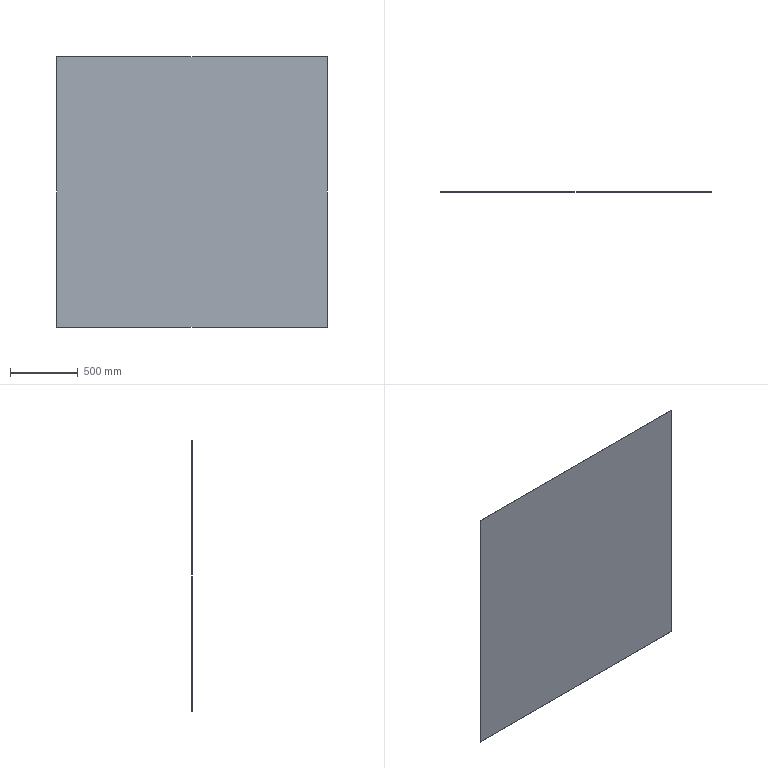Part | STEP file | Ground | 1 solid | 6 faces | box 2000 x 2 x 2000 mm | volume 8000000 mm3 | plane 6
STEP:
#1=CARTESIAN_POINT('',(1000.,0.,1000.));
#2=VERTEX_POINT('',#1);
#3=CARTESIAN_POINT('',(1000.,0.,-1000.));
#4=VERTEX_POINT('',#3);
#5=CARTESIAN_POINT('',(1000.,0.,1000.));
#6=DIRECTION('',(0.,0.,-1.));
#7=VECTOR('',#6,1000.);
#8=LINE('',#5,#7);
#9=EDGE_CURVE('',#2,#4,#8,.T.);
#10=ORIENTED_EDGE('',*,*,#9,.T.);
#11=CARTESIAN_POINT('',(1000.,2.,-1000.));
#12=VERTEX_POINT('',#11);
#13=CARTESIAN_POINT('',(1000.,2.,-1000.));
#14=DIRECTION('',(0.,-1.,0.));
#15=VECTOR('',#14,1000.);
#16=LINE('',#13,#15);
#17=EDGE_CURVE('',#12,#4,#16,.T.);
#18=ORIENTED_EDGE('',*,*,#17,.F.);
#19=CARTESIAN_POINT('',(1000.,2.,1000.));
#20=VERTEX_POINT('',#19);
#21=CARTESIAN_POINT('',(1000.,2.,1000.));
#22=DIRECTION('',(0.,0.,-1.));
#23=VECTOR('',#22,1000.);
#24=LINE('',#21,#23);
#25=EDGE_CURVE('',#20,#12,#24,.T.);
#26=ORIENTED_EDGE('',*,*,#25,.F.);
#27=CARTESIAN_POINT('',(1000.,2.,1000.));
#28=DIRECTION('',(0.,-1.,0.));
#29=VECTOR('',#28,1000.);
#30=LINE('',#27,#29);
#31=EDGE_CURVE('',#20,#2,#30,.T.);
#32=ORIENTED_EDGE('',*,*,#31,.T.);
#33=EDGE_LOOP('',(#10,#18,#26,#32));
#34=FACE_OUTER_BOUND('',#33,.T.);
#35=CARTESIAN_POINT('',(1000.,2.,1000.));
#36=DIRECTION('',(-1.,0.,0.));
#37=DIRECTION('',(0.,0.,1.));
#38=AXIS2_PLACEMENT_3D('',#35,#36,#37);
#39=PLANE('',#38);
#40=ADVANCED_FACE('',(#34),#39,.F.);
#41=CARTESIAN_POINT('',(-1000.,0.,-1000.));
#42=VERTEX_POINT('',#41);
#43=CARTESIAN_POINT('',(-1000.,0.,-1000.));
#44=DIRECTION('',(-1.,0.,0.));
#45=VECTOR('',#44,1000.);
#46=LINE('',#43,#45);
#47=EDGE_CURVE('',#4,#42,#46,.T.);
#48=ORIENTED_EDGE('',*,*,#47,.T.);
#49=CARTESIAN_POINT('',(-1000.,2.,-1000.));
#50=VERTEX_POINT('',#49);
#51=CARTESIAN_POINT('',(-1000.,2.,-1000.));
#52=DIRECTION('',(0.,-1.,0.));
#53=VECTOR('',#52,1000.);
#54=LINE('',#51,#53);
#55=EDGE_CURVE('',#50,#42,#54,.T.);
#56=ORIENTED_EDGE('',*,*,#55,.F.);
#57=CARTESIAN_POINT('',(-1000.,2.,-1000.));
#58=DIRECTION('',(-1.,0.,0.));
#59=VECTOR('',#58,1000.);
#60=LINE('',#57,#59);
#61=EDGE_CURVE('',#12,#50,#60,.T.);
#62=ORIENTED_EDGE('',*,*,#61,.F.);
#63=ORIENTED_EDGE('',*,*,#17,.T.);
#64=EDGE_LOOP('',(#48,#56,#62,#63));
#65=FACE_OUTER_BOUND('',#64,.T.);
#66=CARTESIAN_POINT('',(-1000.,2.,-1000.));
#67=DIRECTION('',(0.,0.,1.));
#68=DIRECTION('',(1.,0.,0.));
#69=AXIS2_PLACEMENT_3D('',#66,#67,#68);
#70=PLANE('',#69);
#71=ADVANCED_FACE('',(#65),#70,.F.);
#72=CARTESIAN_POINT('',(-1000.,0.,1000.));
#73=VERTEX_POINT('',#72);
#74=CARTESIAN_POINT('',(-1000.,0.,1000.));
#75=DIRECTION('',(0.,0.,1.));
#76=VECTOR('',#75,1000.);
#77=LINE('',#74,#76);
#78=EDGE_CURVE('',#42,#73,#77,.T.);
#79=ORIENTED_EDGE('',*,*,#78,.T.);
#80=CARTESIAN_POINT('',(-1000.,2.,1000.));
#81=VERTEX_POINT('',#80);
#82=CARTESIAN_POINT('',(-1000.,2.,1000.));
#83=DIRECTION('',(0.,-1.,0.));
#84=VECTOR('',#83,1000.);
#85=LINE('',#82,#84);
#86=EDGE_CURVE('',#81,#73,#85,.T.);
#87=ORIENTED_EDGE('',*,*,#86,.F.);
#88=CARTESIAN_POINT('',(-1000.,2.,1000.));
#89=DIRECTION('',(0.,0.,1.));
#90=VECTOR('',#89,1000.);
#91=LINE('',#88,#90);
#92=EDGE_CURVE('',#50,#81,#91,.T.);
#93=ORIENTED_EDGE('',*,*,#92,.F.);
#94=ORIENTED_EDGE('',*,*,#55,.T.);
#95=EDGE_LOOP('',(#79,#87,#93,#94));
#96=FACE_OUTER_BOUND('',#95,.T.);
#97=CARTESIAN_POINT('',(-1000.,2.,1000.));
#98=DIRECTION('',(1.,0.,0.));
#99=DIRECTION('',(0.,0.,-1.));
#100=AXIS2_PLACEMENT_3D('',#97,#98,#99);
#101=PLANE('',#100);
#102=ADVANCED_FACE('',(#96),#101,.F.);
#103=CARTESIAN_POINT('',(-1000.,0.,1000.));
#104=DIRECTION('',(1.,0.,0.));
#105=VECTOR('',#104,1000.);
#106=LINE('',#103,#105);
#107=EDGE_CURVE('',#73,#2,#106,.T.);
#108=ORIENTED_EDGE('',*,*,#107,.T.);
#109=ORIENTED_EDGE('',*,*,#31,.F.);
#110=CARTESIAN_POINT('',(-1000.,2.,1000.));
#111=DIRECTION('',(1.,0.,0.));
#112=VECTOR('',#111,1000.);
#113=LINE('',#110,#112);
#114=EDGE_CURVE('',#81,#20,#113,.T.);
#115=ORIENTED_EDGE('',*,*,#114,.F.);
#116=ORIENTED_EDGE('',*,*,#86,.T.);
#117=EDGE_LOOP('',(#108,#109,#115,#116));
#118=FACE_OUTER_BOUND('',#117,.T.);
#119=CARTESIAN_POINT('',(-1000.,2.,1000.));
#120=DIRECTION('',(0.,0.,-1.));
#121=DIRECTION('',(-1.,0.,0.));
#122=AXIS2_PLACEMENT_3D('',#119,#120,#121);
#123=PLANE('',#122);
#124=ADVANCED_FACE('',(#118),#123,.F.);
#125=ORIENTED_EDGE('',*,*,#25,.T.);
#126=ORIENTED_EDGE('',*,*,#61,.T.);
#127=ORIENTED_EDGE('',*,*,#92,.T.);
#128=ORIENTED_EDGE('',*,*,#114,.T.);
#129=EDGE_LOOP('',(#125,#126,#127,#128));
#130=FACE_OUTER_BOUND('',#129,.T.);
#131=CARTESIAN_POINT('',(0.,2.,0.));
#132=DIRECTION('',(0.,-1.,0.));
#133=DIRECTION('',(0.,0.,-1.));
#134=AXIS2_PLACEMENT_3D('',#131,#132,#133);
#135=PLANE('',#134);
#136=ADVANCED_FACE('',(#130),#135,.F.);
#137=ORIENTED_EDGE('',*,*,#9,.F.);
#138=ORIENTED_EDGE('',*,*,#107,.F.);
#139=ORIENTED_EDGE('',*,*,#78,.F.);
#140=ORIENTED_EDGE('',*,*,#47,.F.);
#141=EDGE_LOOP('',(#137,#138,#139,#140));
#142=FACE_OUTER_BOUND('',#141,.T.);
#143=CARTESIAN_POINT('',(0.,0.,0.));
#144=DIRECTION('',(0.,-1.,0.));
#145=DIRECTION('',(0.,0.,-1.));
#146=AXIS2_PLACEMENT_3D('',#143,#144,#145);
#147=PLANE('',#146);
#148=ADVANCED_FACE('',(#142),#147,.T.);
#149=CLOSED_SHELL('',(#40,#71,#102,#124,#136,#148));
#150=MANIFOLD_SOLID_BREP('',#149);
#151=CARTESIAN_POINT('',(0.,0.,0.));
#152=DIRECTION('',(0.,0.,1.));
#153=DIRECTION('',(1.,0.,0.));
#154=AXIS2_PLACEMENT_3D('',#151,#152,#153);
#155=(LENGTH_UNIT()NAMED_UNIT(*)SI_UNIT(.MILLI.,.METRE.));
#156=UNCERTAINTY_MEASURE_WITH_UNIT(LENGTH_MEASURE(0.00001),#155,'','');
#157=(NAMED_UNIT(*)PLANE_ANGLE_UNIT()SI_UNIT($,.RADIAN.));
#158=(NAMED_UNIT(*)SI_UNIT($,.STERADIAN.)SOLID_ANGLE_UNIT());
#159=(GEOMETRIC_REPRESENTATION_CONTEXT(3)GLOBAL_UNCERTAINTY_ASSIGNED_CONTEXT((#156))GLOBAL_UNIT_ASSIGNED_CONTEXT((#155,#157,#158))REPRESENTATION_CONTEXT('',''));
#160=ADVANCED_BREP_SHAPE_REPRESENTATION('',(#150,#154),#159);